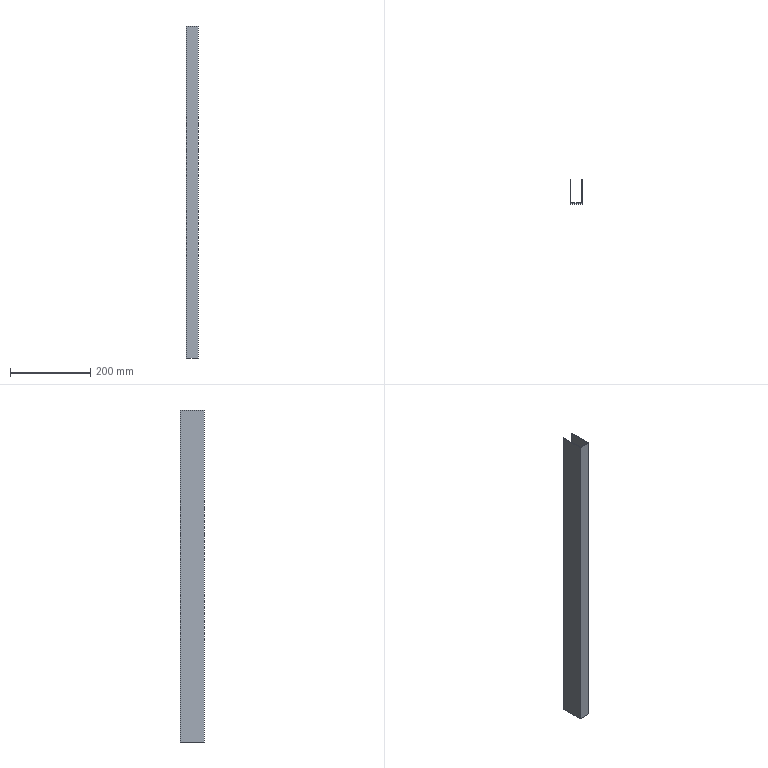Part | SolidWorks | features Extrusion 1, Shell 1 | 1 solid | 10 faces | box 30 x 60 x 830 mm | volume 242360 mm3 | plane 10
STEP:
#1=CARTESIAN_POINT('',(13.,30.,415.));
#2=VERTEX_POINT('',#1);
#3=CARTESIAN_POINT('',(13.,30.,-415.));
#4=VERTEX_POINT('',#3);
#5=CARTESIAN_POINT('',(13.,30.,415.));
#6=DIRECTION('',(0.,0.,-1.));
#7=VECTOR('',#6,1000.);
#8=LINE('',#5,#7);
#9=EDGE_CURVE('',#2,#4,#8,.T.);
#10=ORIENTED_EDGE('',*,*,#9,.F.);
#11=CARTESIAN_POINT('',(15.,30.,415.));
#12=VERTEX_POINT('',#11);
#13=CARTESIAN_POINT('',(-15.,30.,415.));
#14=DIRECTION('',(-1.,0.,0.));
#15=VECTOR('',#14,1000.);
#16=LINE('',#13,#15);
#17=EDGE_CURVE('',#12,#2,#16,.T.);
#18=ORIENTED_EDGE('',*,*,#17,.F.);
#19=CARTESIAN_POINT('',(15.,30.,-415.));
#20=VERTEX_POINT('',#19);
#21=CARTESIAN_POINT('',(15.,30.,415.));
#22=DIRECTION('',(0.,0.,-1.));
#23=VECTOR('',#22,1000.);
#24=LINE('',#21,#23);
#25=EDGE_CURVE('',#12,#20,#24,.T.);
#26=ORIENTED_EDGE('',*,*,#25,.T.);
#27=CARTESIAN_POINT('',(-15.,30.,-415.));
#28=DIRECTION('',(-1.,0.,0.));
#29=VECTOR('',#28,1000.);
#30=LINE('',#27,#29);
#31=EDGE_CURVE('',#20,#4,#30,.T.);
#32=ORIENTED_EDGE('',*,*,#31,.T.);
#33=EDGE_LOOP('',(#10,#18,#26,#32));
#34=FACE_OUTER_BOUND('',#33,.T.);
#35=CARTESIAN_POINT('',(-15.,30.,415.));
#36=DIRECTION('',(0.,-1.,0.));
#37=DIRECTION('',(0.,0.,-1.));
#38=AXIS2_PLACEMENT_3D('',#35,#36,#37);
#39=PLANE('',#38);
#40=ADVANCED_FACE('',(#34),#39,.F.);
#41=CARTESIAN_POINT('',(13.,-28.,415.));
#42=VERTEX_POINT('',#41);
#43=CARTESIAN_POINT('',(13.,0.,415.));
#44=DIRECTION('',(0.,1.,0.));
#45=VECTOR('',#44,1000.);
#46=LINE('',#43,#45);
#47=EDGE_CURVE('',#42,#2,#46,.T.);
#48=ORIENTED_EDGE('',*,*,#47,.F.);
#49=CARTESIAN_POINT('',(-13.,-28.,415.));
#50=VERTEX_POINT('',#49);
#51=CARTESIAN_POINT('',(0.,-28.,415.));
#52=DIRECTION('',(1.,0.,0.));
#53=VECTOR('',#52,1000.);
#54=LINE('',#51,#53);
#55=EDGE_CURVE('',#50,#42,#54,.T.);
#56=ORIENTED_EDGE('',*,*,#55,.F.);
#57=CARTESIAN_POINT('',(-13.,30.,415.));
#58=VERTEX_POINT('',#57);
#59=CARTESIAN_POINT('',(-13.,0.,415.));
#60=DIRECTION('',(0.,-1.,0.));
#61=VECTOR('',#60,1000.);
#62=LINE('',#59,#61);
#63=EDGE_CURVE('',#58,#50,#62,.T.);
#64=ORIENTED_EDGE('',*,*,#63,.F.);
#65=CARTESIAN_POINT('',(-15.,30.,415.));
#66=VERTEX_POINT('',#65);
#67=CARTESIAN_POINT('',(-15.,30.,415.));
#68=DIRECTION('',(-1.,0.,0.));
#69=VECTOR('',#68,1000.);
#70=LINE('',#67,#69);
#71=EDGE_CURVE('',#58,#66,#70,.T.);
#72=ORIENTED_EDGE('',*,*,#71,.T.);
#73=CARTESIAN_POINT('',(-15.,-30.,415.));
#74=VERTEX_POINT('',#73);
#75=CARTESIAN_POINT('',(-15.,-30.,415.));
#76=DIRECTION('',(0.,-1.,0.));
#77=VECTOR('',#76,1000.);
#78=LINE('',#75,#77);
#79=EDGE_CURVE('',#66,#74,#78,.T.);
#80=ORIENTED_EDGE('',*,*,#79,.T.);
#81=CARTESIAN_POINT('',(15.,-30.,415.));
#82=VERTEX_POINT('',#81);
#83=CARTESIAN_POINT('',(-15.,-30.,415.));
#84=DIRECTION('',(1.,0.,0.));
#85=VECTOR('',#84,1000.);
#86=LINE('',#83,#85);
#87=EDGE_CURVE('',#74,#82,#86,.T.);
#88=ORIENTED_EDGE('',*,*,#87,.T.);
#89=CARTESIAN_POINT('',(15.,-30.,415.));
#90=DIRECTION('',(0.,1.,0.));
#91=VECTOR('',#90,1000.);
#92=LINE('',#89,#91);
#93=EDGE_CURVE('',#82,#12,#92,.T.);
#94=ORIENTED_EDGE('',*,*,#93,.T.);
#95=ORIENTED_EDGE('',*,*,#17,.T.);
#96=EDGE_LOOP('',(#48,#56,#64,#72,#80,#88,#94,#95));
#97=FACE_OUTER_BOUND('',#96,.T.);
#98=CARTESIAN_POINT('',(0.,0.,415.));
#99=DIRECTION('',(0.,0.,-1.));
#100=DIRECTION('',(-1.,0.,0.));
#101=AXIS2_PLACEMENT_3D('',#98,#99,#100);
#102=PLANE('',#101);
#103=ADVANCED_FACE('',(#97),#102,.F.);
#104=CARTESIAN_POINT('',(-13.,-28.,-415.));
#105=VERTEX_POINT('',#104);
#106=CARTESIAN_POINT('',(13.,-28.,-415.));
#107=VERTEX_POINT('',#106);
#108=CARTESIAN_POINT('',(0.,-28.,-415.));
#109=DIRECTION('',(1.,0.,0.));
#110=VECTOR('',#109,1000.);
#111=LINE('',#108,#110);
#112=EDGE_CURVE('',#105,#107,#111,.T.);
#113=ORIENTED_EDGE('',*,*,#112,.T.);
#114=CARTESIAN_POINT('',(13.,0.,-415.));
#115=DIRECTION('',(0.,1.,0.));
#116=VECTOR('',#115,1000.);
#117=LINE('',#114,#116);
#118=EDGE_CURVE('',#107,#4,#117,.T.);
#119=ORIENTED_EDGE('',*,*,#118,.T.);
#120=ORIENTED_EDGE('',*,*,#31,.F.);
#121=CARTESIAN_POINT('',(15.,-30.,-415.));
#122=VERTEX_POINT('',#121);
#123=CARTESIAN_POINT('',(15.,-30.,-415.));
#124=DIRECTION('',(0.,1.,0.));
#125=VECTOR('',#124,1000.);
#126=LINE('',#123,#125);
#127=EDGE_CURVE('',#122,#20,#126,.T.);
#128=ORIENTED_EDGE('',*,*,#127,.F.);
#129=CARTESIAN_POINT('',(-15.,-30.,-415.));
#130=VERTEX_POINT('',#129);
#131=CARTESIAN_POINT('',(-15.,-30.,-415.));
#132=DIRECTION('',(1.,0.,0.));
#133=VECTOR('',#132,1000.);
#134=LINE('',#131,#133);
#135=EDGE_CURVE('',#130,#122,#134,.T.);
#136=ORIENTED_EDGE('',*,*,#135,.F.);
#137=CARTESIAN_POINT('',(-15.,30.,-415.));
#138=VERTEX_POINT('',#137);
#139=CARTESIAN_POINT('',(-15.,-30.,-415.));
#140=DIRECTION('',(0.,-1.,0.));
#141=VECTOR('',#140,1000.);
#142=LINE('',#139,#141);
#143=EDGE_CURVE('',#138,#130,#142,.T.);
#144=ORIENTED_EDGE('',*,*,#143,.F.);
#145=CARTESIAN_POINT('',(-13.,30.,-415.));
#146=VERTEX_POINT('',#145);
#147=CARTESIAN_POINT('',(-15.,30.,-415.));
#148=DIRECTION('',(-1.,0.,0.));
#149=VECTOR('',#148,1000.);
#150=LINE('',#147,#149);
#151=EDGE_CURVE('',#146,#138,#150,.T.);
#152=ORIENTED_EDGE('',*,*,#151,.F.);
#153=CARTESIAN_POINT('',(-13.,0.,-415.));
#154=DIRECTION('',(0.,-1.,0.));
#155=VECTOR('',#154,1000.);
#156=LINE('',#153,#155);
#157=EDGE_CURVE('',#146,#105,#156,.T.);
#158=ORIENTED_EDGE('',*,*,#157,.T.);
#159=EDGE_LOOP('',(#113,#119,#120,#128,#136,#144,#152,#158));
#160=FACE_OUTER_BOUND('',#159,.T.);
#161=CARTESIAN_POINT('',(0.,0.,-415.));
#162=DIRECTION('',(0.,0.,-1.));
#163=DIRECTION('',(-1.,0.,0.));
#164=AXIS2_PLACEMENT_3D('',#161,#162,#163);
#165=PLANE('',#164);
#166=ADVANCED_FACE('',(#160),#165,.T.);
#167=ORIENTED_EDGE('',*,*,#127,.T.);
#168=ORIENTED_EDGE('',*,*,#25,.F.);
#169=ORIENTED_EDGE('',*,*,#93,.F.);
#170=CARTESIAN_POINT('',(15.,-30.,415.));
#171=DIRECTION('',(0.,0.,-1.));
#172=VECTOR('',#171,1000.);
#173=LINE('',#170,#172);
#174=EDGE_CURVE('',#82,#122,#173,.T.);
#175=ORIENTED_EDGE('',*,*,#174,.T.);
#176=EDGE_LOOP('',(#167,#168,#169,#175));
#177=FACE_OUTER_BOUND('',#176,.T.);
#178=CARTESIAN_POINT('',(15.,-30.,415.));
#179=DIRECTION('',(-1.,0.,0.));
#180=DIRECTION('',(0.,0.,1.));
#181=AXIS2_PLACEMENT_3D('',#178,#179,#180);
#182=PLANE('',#181);
#183=ADVANCED_FACE('',(#177),#182,.F.);
#184=ORIENTED_EDGE('',*,*,#71,.F.);
#185=CARTESIAN_POINT('',(-13.,30.,415.));
#186=DIRECTION('',(0.,0.,-1.));
#187=VECTOR('',#186,1000.);
#188=LINE('',#185,#187);
#189=EDGE_CURVE('',#58,#146,#188,.T.);
#190=ORIENTED_EDGE('',*,*,#189,.T.);
#191=ORIENTED_EDGE('',*,*,#151,.T.);
#192=CARTESIAN_POINT('',(-15.,30.,415.));
#193=DIRECTION('',(0.,0.,-1.));
#194=VECTOR('',#193,1000.);
#195=LINE('',#192,#194);
#196=EDGE_CURVE('',#66,#138,#195,.T.);
#197=ORIENTED_EDGE('',*,*,#196,.F.);
#198=EDGE_LOOP('',(#184,#190,#191,#197));
#199=FACE_OUTER_BOUND('',#198,.T.);
#200=CARTESIAN_POINT('',(-15.,30.,415.));
#201=DIRECTION('',(0.,-1.,0.));
#202=DIRECTION('',(0.,0.,-1.));
#203=AXIS2_PLACEMENT_3D('',#200,#201,#202);
#204=PLANE('',#203);
#205=ADVANCED_FACE('',(#199),#204,.F.);
#206=ORIENTED_EDGE('',*,*,#143,.T.);
#207=CARTESIAN_POINT('',(-15.,-30.,415.));
#208=DIRECTION('',(0.,0.,-1.));
#209=VECTOR('',#208,1000.);
#210=LINE('',#207,#209);
#211=EDGE_CURVE('',#74,#130,#210,.T.);
#212=ORIENTED_EDGE('',*,*,#211,.F.);
#213=ORIENTED_EDGE('',*,*,#79,.F.);
#214=ORIENTED_EDGE('',*,*,#196,.T.);
#215=EDGE_LOOP('',(#206,#212,#213,#214));
#216=FACE_OUTER_BOUND('',#215,.T.);
#217=CARTESIAN_POINT('',(-15.,-30.,415.));
#218=DIRECTION('',(1.,0.,0.));
#219=DIRECTION('',(0.,0.,-1.));
#220=AXIS2_PLACEMENT_3D('',#217,#218,#219);
#221=PLANE('',#220);
#222=ADVANCED_FACE('',(#216),#221,.F.);
#223=ORIENTED_EDGE('',*,*,#135,.T.);
#224=ORIENTED_EDGE('',*,*,#174,.F.);
#225=ORIENTED_EDGE('',*,*,#87,.F.);
#226=ORIENTED_EDGE('',*,*,#211,.T.);
#227=EDGE_LOOP('',(#223,#224,#225,#226));
#228=FACE_OUTER_BOUND('',#227,.T.);
#229=CARTESIAN_POINT('',(-15.,-30.,415.));
#230=DIRECTION('',(0.,1.,0.));
#231=DIRECTION('',(0.,0.,1.));
#232=AXIS2_PLACEMENT_3D('',#229,#230,#231);
#233=PLANE('',#232);
#234=ADVANCED_FACE('',(#228),#233,.F.);
#235=ORIENTED_EDGE('',*,*,#118,.F.);
#236=CARTESIAN_POINT('',(13.,-28.,415.));
#237=DIRECTION('',(0.,0.,-1.));
#238=VECTOR('',#237,1000.);
#239=LINE('',#236,#238);
#240=EDGE_CURVE('',#42,#107,#239,.T.);
#241=ORIENTED_EDGE('',*,*,#240,.F.);
#242=ORIENTED_EDGE('',*,*,#47,.T.);
#243=ORIENTED_EDGE('',*,*,#9,.T.);
#244=EDGE_LOOP('',(#235,#241,#242,#243));
#245=FACE_OUTER_BOUND('',#244,.T.);
#246=CARTESIAN_POINT('',(13.,-30.,415.));
#247=DIRECTION('',(-1.,0.,0.));
#248=DIRECTION('',(0.,0.,1.));
#249=AXIS2_PLACEMENT_3D('',#246,#247,#248);
#250=PLANE('',#249);
#251=ADVANCED_FACE('',(#245),#250,.T.);
#252=ORIENTED_EDGE('',*,*,#157,.F.);
#253=ORIENTED_EDGE('',*,*,#189,.F.);
#254=ORIENTED_EDGE('',*,*,#63,.T.);
#255=CARTESIAN_POINT('',(-13.,-28.,415.));
#256=DIRECTION('',(0.,0.,-1.));
#257=VECTOR('',#256,1000.);
#258=LINE('',#255,#257);
#259=EDGE_CURVE('',#50,#105,#258,.T.);
#260=ORIENTED_EDGE('',*,*,#259,.T.);
#261=EDGE_LOOP('',(#252,#253,#254,#260));
#262=FACE_OUTER_BOUND('',#261,.T.);
#263=CARTESIAN_POINT('',(-13.,-30.,415.));
#264=DIRECTION('',(1.,0.,0.));
#265=DIRECTION('',(0.,0.,-1.));
#266=AXIS2_PLACEMENT_3D('',#263,#264,#265);
#267=PLANE('',#266);
#268=ADVANCED_FACE('',(#262),#267,.T.);
#269=ORIENTED_EDGE('',*,*,#112,.F.);
#270=ORIENTED_EDGE('',*,*,#259,.F.);
#271=ORIENTED_EDGE('',*,*,#55,.T.);
#272=ORIENTED_EDGE('',*,*,#240,.T.);
#273=EDGE_LOOP('',(#269,#270,#271,#272));
#274=FACE_OUTER_BOUND('',#273,.T.);
#275=CARTESIAN_POINT('',(-15.,-28.,415.));
#276=DIRECTION('',(0.,1.,0.));
#277=DIRECTION('',(0.,0.,1.));
#278=AXIS2_PLACEMENT_3D('',#275,#276,#277);
#279=PLANE('',#278);
#280=ADVANCED_FACE('',(#274),#279,.T.);
#281=CLOSED_SHELL('',(#40,#103,#166,#183,#205,#222,#234,#251,#268,#280));
#282=MANIFOLD_SOLID_BREP('',#281);
#283=CARTESIAN_POINT('',(0.,0.,0.));
#284=DIRECTION('',(0.,0.,1.));
#285=DIRECTION('',(1.,0.,0.));
#286=AXIS2_PLACEMENT_3D('',#283,#284,#285);
#287=(LENGTH_UNIT()NAMED_UNIT(*)SI_UNIT(.MILLI.,.METRE.));
#288=UNCERTAINTY_MEASURE_WITH_UNIT(LENGTH_MEASURE(0.00001),#287,'','');
#289=(NAMED_UNIT(*)PLANE_ANGLE_UNIT()SI_UNIT($,.RADIAN.));
#290=(NAMED_UNIT(*)SI_UNIT($,.STERADIAN.)SOLID_ANGLE_UNIT());
#291=(GEOMETRIC_REPRESENTATION_CONTEXT(3)GLOBAL_UNCERTAINTY_ASSIGNED_CONTEXT((#288))GLOBAL_UNIT_ASSIGNED_CONTEXT((#287,#289,#290))REPRESENTATION_CONTEXT('',''));
#292=ADVANCED_BREP_SHAPE_REPRESENTATION('',(#282,#286),#291);